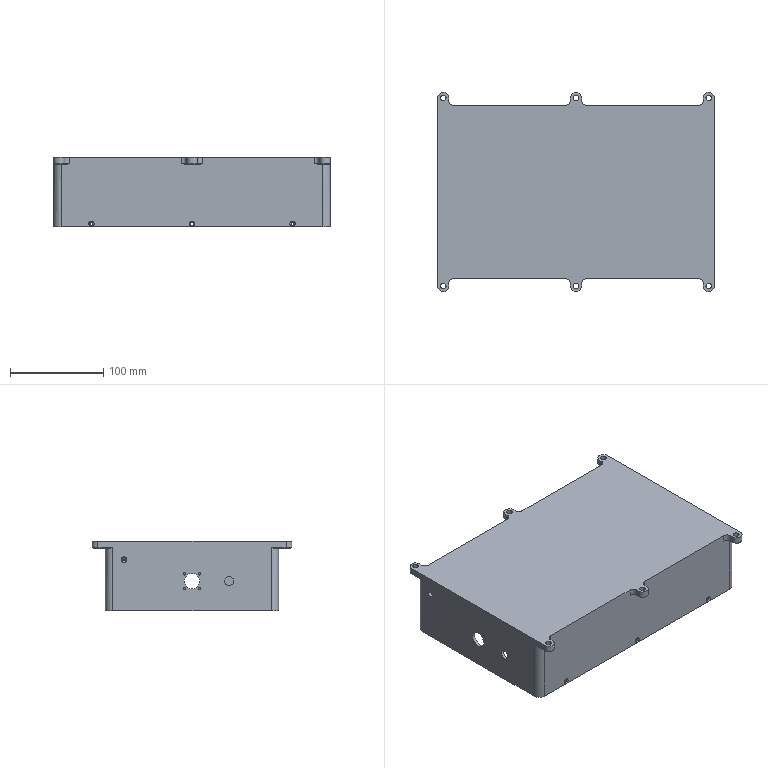NC program | NX | posted with a generic post | part box 297 x 214 x 75 mm
Whole program:
N10 G17 G21 G94 G90
(CAVITY_MILL , TOOL : D10JING)
N12 T14 M6
N14 G54
N16 G17 G0 G90 X-129.632 Y102.849 B0. C0. S9500 M3
N18 G43 Z30. H14
N20 Z-1.
N22 G94 G1 X-131.013 Y102.026 F1600.
N24 G3 X-131.501 Y101.153 R1.
N26 G1 X-131.5 Y101.
N28 Y98.
N30 X-128.347
N32 G3 X-127.481 Y98.5 R1.
N34 G1 X-126.615 Y100.
N36 G0 X-129.632 Y102.849 Z-2.
N38 G1 X-131.013 Y102.026
N40 G3 X-131.501 Y101.153 R1.
N42 G1 X-131.5 Y101.
N44 Y98.
N46 X-128.347
N48 G3 X-127.481 Y98.5 R1.
N50 G1 X-126.615 Y100.
N52 G0 X-129.632 Y102.849 Z-3.
N54 G1 X-131.013 Y102.026
N56 G3 X-131.501 Y101.153 R1.
N58 G1 X-131.5 Y101.
N60 Y98.
N62 X-128.347
N64 G3 X-127.481 Y98.5 R1.
N66 G1 X-126.615 Y100.
N68 G0 X-129.632 Y102.849 Z-4.
N70 G1 X-131.013 Y102.026
N72 G3 X-131.501 Y101.153 R1.
N74 G1 X-131.5 Y101.
N76 Y98.
N78 X-128.347
N80 G3 X-127.481 Y98.5 R1.
N82 G1 X-126.615 Y100.
N84 G0 X-129.632 Y102.849 Z-5.
N86 G1 X-131.013 Y102.026
N88 G3 X-131.501 Y101.153 R1.
N90 G1 X-131.5 Y101.
N92 Y98.
N94 X-128.347
N96 G3 X-127.481 Y98.5 R1.
N98 G1 X-126.615 Y100.
N100 G0 X-129.632 Y102.849 Z-6.
N102 G1 X-131.013 Y102.026
N104 G3 X-131.501 Y101.153 R1.
N106 G1 X-131.5 Y101.
N108 Y98.
N110 X-128.347
N112 G3 X-127.481 Y98.5 R1.
N114 G1 X-126.615 Y100.
N116 G0 X-129.632 Y102.849 Z-7.
N118 G1 X-131.013 Y102.026
N120 G3 X-131.501 Y101.153 R1.
N122 G1 X-131.5 Y101.
N124 Y98.
N126 X-128.347
N128 G3 X-127.481 Y98.5 R1.
N130 G1 X-126.615 Y100.
N132 G0 X-129.632 Y102.849 Z-8.
N134 G1 X-131.013 Y102.026
N136 G3 X-131.501 Y101.153 R1.
N138 G1 X-131.5 Y101.
N140 Y98.
N142 X-128.347
N144 G3 X-127.481 Y98.5 R1.
N146 G1 X-126.615 Y100.
N148 G0 X-129.632 Y102.849 Z-9.
N150 G1 X-131.013 Y102.026
N152 G3 X-131.501 Y101.153 R1.
N154 G1 X-131.5 Y101.
N156 Y98.
N158 X-128.347
N160 G3 X-127.481 Y98.5 R1.
N162 G1 X-126.615 Y100.
N164 G0 X-129.632 Y102.849 Z-10.
N166 G1 X-131.013 Y102.026
N168 G3 X-131.501 Y101.153 R1.
N170 G1 X-131.5 Y101.
N172 Y98.
N174 X-128.347
N176 G3 X-127.481 Y98.5 R1.
N178 G1 X-126.615 Y100.
N180 G0 Z30.
N182 X-15.885
N184 Z-1.
N186 G1 X-15.019 Y98.5
N188 G3 X-14.153 Y98. R1.
N190 G1 X-11.
N192 Y101.
N194 X-10.999 Y101.153
N196 G3 X-11.487 Y102.026 R1.
N198 G1 X-12.868 Y102.849
N200 G0 X-15.885 Y100. Z-2.
N202 G1 X-15.019 Y98.5
N204 G3 X-14.153 Y98. R1.
N206 G1 X-11.
N208 Y101.
N210 X-10.999 Y101.153
N212 G3 X-11.487 Y102.026 R1.
N214 G1 X-12.868 Y102.849
N216 G0 X-15.885 Y100. Z-3.
N218 G1 X-15.019 Y98.5
N220 G3 X-14.153 Y98. R1.
N222 G1 X-11.
N224 Y101.
N226 X-10.999 Y101.153
N228 G3 X-11.487 Y102.026 R1.
N230 G1 X-12.868 Y102.849
N232 G0 X-15.885 Y100. Z-4.
N234 G1 X-15.019 Y98.5
N236 G3 X-14.153 Y98. R1.
N238 G1 X-11.
N240 Y101.
N242 X-10.999 Y101.153
N244 G3 X-11.487 Y102.026 R1.
N246 G1 X-12.868 Y102.849
N248 G0 X-15.885 Y100. Z-5.
N250 G1 X-15.019 Y98.5
N252 G3 X-14.153 Y98. R1.
N254 G1 X-11.
N256 Y101.
N258 X-10.999 Y101.153
N260 G3 X-11.487 Y102.026 R1.
N262 G1 X-12.868 Y102.849
N264 G0 X-15.885 Y100. Z-6.
N266 G1 X-15.019 Y98.5
N268 G3 X-14.153 Y98. R1.
N270 G1 X-11.
N272 Y101.
N274 X-10.999 Y101.153
N276 G3 X-11.487 Y102.026 R1.
N278 G1 X-12.868 Y102.849
N280 G0 X-15.885 Y100. Z-7.
N282 G1 X-15.019 Y98.5
N284 G3 X-14.153 Y98. R1.
N286 G1 X-11.
N288 Y101.
N290 X-10.999 Y101.153
N292 G3 X-11.487 Y102.026 R1.
N294 G1 X-12.868 Y102.849
N296 G0 X-15.885 Y100. Z-8.
N298 G1 X-15.019 Y98.5
N300 G3 X-14.153 Y98. R1.
N302 G1 X-11.
N304 Y101.
N306 X-10.999 Y101.153
N308 G3 X-11.487 Y102.026 R1.
N310 G1 X-12.868 Y102.849
N312 G0 X-15.885 Y100. Z-9.
N314 G1 X-15.019 Y98.5
N316 G3 X-14.153 Y98. R1.
N318 G1 X-11.
N320 Y101.
N322 X-10.999 Y101.153
N324 G3 X-11.487 Y102.026 R1.
N326 G1 X-12.868 Y102.849
N328 G0 X-15.885 Y100. Z-10.
N330 G1 X-15.019 Y98.5
N332 G3 X-14.153 Y98. R1.
N334 G1 X-11.
N336 Y101.
N338 X-10.999 Y101.153
N340 G3 X-11.487 Y102.026 R1.
N342 G1 X-12.868 Y102.849
N344 G0 Z30.
N346 X12.868
N348 Z-1.
N350 G1 X11.487 Y102.026
N352 G3 X10.999 Y101.153 R1.
N354 G1 X11. Y101.
N356 Y98.
N358 X14.153
N360 G3 X15.019 Y98.5 R1.
N362 G1 X15.885 Y100.
N364 G0 X12.868 Y102.849 Z-2.
N366 G1 X11.487 Y102.026
N368 G3 X10.999 Y101.153 R1.
N370 G1 X11. Y101.
N372 Y98.
N374 X14.153
N376 G3 X15.019 Y98.5 R1.
N378 G1 X15.885 Y100.
N380 G0 X12.868 Y102.849 Z-3.
N382 G1 X11.487 Y102.026
N384 G3 X10.999 Y101.153 R1.
N386 G1 X11. Y101.
N388 Y98.
N390 X14.153
N392 G3 X15.019 Y98.5 R1.
N394 G1 X15.885 Y100.
N396 G0 X12.868 Y102.849 Z-4.
N398 G1 X11.487 Y102.026
N400 G3 X10.999 Y101.153 R1.
N402 G1 X11. Y101.
N404 Y98.
N406 X14.153
N408 G3 X15.019 Y98.5 R1.
N410 G1 X15.885 Y100.
N412 G0 X12.868 Y102.849 Z-5.
N414 G1 X11.487 Y102.026
N416 G3 X10.999 Y101.153 R1.
N418 G1 X11. Y101.
N420 Y98.
N422 X14.153
N424 G3 X15.019 Y98.5 R1.
N426 G1 X15.885 Y100.
N428 G0 X12.868 Y102.849 Z-6.
N430 G1 X11.487 Y102.026
N432 G3 X10.999 Y101.153 R1.
N434 G1 X11. Y101.
N436 Y98.
N438 X14.153
N440 G3 X15.019 Y98.5 R1.
N442 G1 X15.885 Y100.
N444 G0 X12.868 Y102.849 Z-7.
N446 G1 X11.487 Y102.026
N448 G3 X10.999 Y101.153 R1.
N450 G1 X11. Y101.
N452 Y98.
N454 X14.153
N456 G3 X15.019 Y98.5 R1.
N458 G1 X15.885 Y100.
N460 G0 X12.868 Y102.849 Z-8.
N462 G1 X11.487 Y102.026
N464 G3 X10.999 Y101.153 R1.
N466 G1 X11. Y101.
N468 Y98.
N470 X14.153
N472 G3 X15.019 Y98.5 R1.
N474 G1 X15.885 Y100.
N476 G0 X12.868 Y102.849 Z-9.
N478 G1 X11.487 Y102.026
N480 G3 X10.999 Y101.153 R1.
N482 G1 X11. Y101.
N484 Y98.
N486 X14.153
N488 G3 X15.019 Y98.5 R1.
N490 G1 X15.885 Y100.
N492 G0 X12.868 Y102.849 Z-10.
N494 G1 X11.487 Y102.026
N496 G3 X10.999 Y101.153 R1.
N498 G1 X11. Y101.
N500 Y98.
N502 X14.153
N504 G3 X15.019 Y98.5 R1.
N506 G1 X15.885 Y100.
N508 G0 Z30.
N510 X126.615
N512 Z-1.
N514 G1 X127.481 Y98.5
N516 G3 X128.347 Y98. R1.
N518 G1 X131.5
N520 Y101.
N522 X131.501 Y101.153
N524 G3 X131.013 Y102.026 R1.
N526 G1 X129.632 Y102.849
N528 G0 X126.615 Y100. Z-2.
N530 G1 X127.481 Y98.5
N532 G3 X128.347 Y98. R1.
N534 G1 X131.5
N536 Y101.
N538 X131.501 Y101.153
N540 G3 X131.013 Y102.026 R1.
N542 G1 X129.632 Y102.849
N544 G0 X126.615 Y100. Z-3.
N546 G1 X127.481 Y98.5
N548 G3 X128.347 Y98. R1.
N550 G1 X131.5
N552 Y101.
N554 X131.501 Y101.153
N556 G3 X131.013 Y102.026 R1.
N558 G1 X129.632 Y102.849
N560 G0 X126.615 Y100. Z-4.
N562 G1 X127.481 Y98.5
N564 G3 X128.347 Y98. R1.
N566 G1 X131.5
N568 Y101.
N570 X131.501 Y101.153
N572 G3 X131.013 Y102.026 R1.
N574 G1 X129.632 Y102.849
N576 G0 X126.615 Y100. Z-5.
N578 G1 X127.481 Y98.5
N580 G3 X128.347 Y98. R1.
N582 G1 X131.5
N584 Y101.
N586 X131.501 Y101.153
N588 G3 X131.013 Y102.026 R1.
N590 G1 X129.632 Y102.849
N592 G0 X126.615 Y100. Z-6.
N594 G1 X127.481 Y98.5
N596 G3 X128.347 Y98. R1.
N598 G1 X131.5
N600 Y101.
N602 X131.501 Y101.153
N604 G3 X131.013 Y102.026 R1.
N606 G1 X129.632 Y102.849
N608 G0 X126.615 Y100. Z-7.
N610 G1 X127.481 Y98.5
N612 G3 X128.347 Y98. R1.
N614 G1 X131.5
N616 Y101.
N618 X131.501 Y101.153
N620 G3 X131.013 Y102.026 R1.
N622 G1 X129.632 Y102.849
N624 G0 X126.615 Y100. Z-8.
N626 G1 X127.481 Y98.5
N628 G3 X128.347 Y98. R1.
N630 G1 X131.5
N632 Y101.
N634 X131.501 Y101.153
N636 G3 X131.013 Y102.026 R1.
N638 G1 X129.632 Y102.849
N640 G0 X126.615 Y100. Z-9.
N642 G1 X127.481 Y98.5
N644 G3 X128.347 Y98. R1.
N646 G1 X131.5
N648 Y101.
N650 X131.501 Y101.153
N652 G3 X131.013 Y102.026 R1.
N654 G1 X129.632 Y102.849
N656 G0 X126.615 Y100. Z-10.
N658 G1 X127.481 Y98.5
N660 G3 X128.347 Y98. R1.
N662 G1 X131.5
N664 Y101.
N666 X131.501 Y101.153
N668 G3 X131.013 Y102.026 R1.
N670 G1 X129.632 Y102.849
N672 G0 Z30.
N674 Y-102.849
N676 Z-1.
N678 G1 X131.013 Y-102.026
N680 G3 X131.501 Y-101.153 R1.
N682 G1 X131.5 Y-101.
N684 Y-98.
N686 X128.347
N688 G3 X127.481 Y-98.5 R1.
N690 G1 X126.615 Y-100.
N692 G0 X129.632 Y-102.849 Z-2.
N694 G1 X131.013 Y-102.026
N696 G3 X131.501 Y-101.153 R1.
N698 G1 X131.5 Y-101.
N700 Y-98.
N702 X128.347
N704 G3 X127.481 Y-98.5 R1.
N706 G1 X126.615 Y-100.
N708 G0 X129.632 Y-102.849 Z-3.
N710 G1 X131.013 Y-102.026
N712 G3 X131.501 Y-101.153 R1.
N714 G1 X131.5 Y-101.
N716 Y-98.
N718 X128.347
N720 G3 X127.481 Y-98.5 R1.
N722 G1 X126.615 Y-100.
N724 G0 X129.632 Y-102.849 Z-4.
N726 G1 X131.013 Y-102.026
N728 G3 X131.501 Y-101.153 R1.
N730 G1 X131.5 Y-101.
N732 Y-98.
N734 X128.347
N736 G3 X127.481 Y-98.5 R1.
N738 G1 X126.615 Y-100.
N740 G0 X129.632 Y-102.849 Z-5.
N742 G1 X131.013 Y-102.026
N744 G3 X131.501 Y-101.153 R1.
N746 G1 X131.5 Y-101.
N748 Y-98.
N750 X128.347
N752 G3 X127.481 Y-98.5 R1.
N754 G1 X126.615 Y-100.
N756 G0 X129.632 Y-102.849 Z-6.
N758 G1 X131.013 Y-102.026
N760 G3 X131.501 Y-101.153 R1.
N762 G1 X131.5 Y-101.
N764 Y-98.
N766 X128.347
N768 G3 X127.481 Y-98.5 R1.
N770 G1 X126.615 Y-100.
N772 G0 X129.632 Y-102.849 Z-7.
N774 G1 X131.013 Y-102.026
N776 G3 X131.501 Y-101.153 R1.
N778 G1 X131.5 Y-101.
N780 Y-98.
N782 X128.347
N784 G3 X127.481 Y-98.5 R1.
N786 G1 X126.615 Y-100.
N788 G0 X129.632 Y-102.849 Z-8.
N790 G1 X131.013 Y-102.026
N792 G3 X131.501 Y-101.153 R1.
N794 G1 X131.5 Y-101.
N796 Y-98.
N798 X128.347
N800 G3 X127.481 Y-98.5 R1.
N802 G1 X126.615 Y-100.
N804 G0 X129.632 Y-102.849 Z-9.
N806 G1 X131.013 Y-102.026
N808 G3 X131.501 Y-101.153 R1.
N810 G1 X131.5 Y-101.
N812 Y-98.
N814 X128.347
N816 G3 X127.481 Y-98.5 R1.
N818 G1 X126.615 Y-100.
N820 G0 X129.632 Y-102.849 Z-10.
N822 G1 X131.013 Y-102.026
N824 G3 X131.501 Y-101.153 R1.
N826 G1 X131.5 Y-101.
N828 Y-98.
N830 X128.347
N832 G3 X127.481 Y-98.5 R1.
N834 G1 X126.615 Y-100.
N836 G0 Z30.
N838 X15.885
N840 Z-1.
N842 G1 X15.019 Y-98.5
N844 G3 X14.153 Y-98. R1.
N846 G1 X11.
N848 Y-101.
N850 X10.999 Y-101.153
N852 G3 X11.487 Y-102.026 R1.
N854 G1 X12.868 Y-102.849
N856 G0 X15.885 Y-100. Z-2.
N858 G1 X15.019 Y-98.5
N860 G3 X14.153 Y-98. R1.
N862 G1 X11.
N864 Y-101.
N866 X10.999 Y-101.153
N868 G3 X11.487 Y-102.026 R1.
N870 G1 X12.868 Y-102.849
N872 G0 X15.885 Y-100. Z-3.
N874 G1 X15.019 Y-98.5
N876 G3 X14.153 Y-98. R1.
N878 G1 X11.
N880 Y-101.
N882 X10.999 Y-101.153
N884 G3 X11.487 Y-102.026 R1.
N886 G1 X12.868 Y-102.849
N888 G0 X15.885 Y-100. Z-4.
N890 G1 X15.019 Y-98.5
N892 G3 X14.153 Y-98. R1.
N894 G1 X11.
N896 Y-101.
N898 X10.999 Y-101.153
N900 G3 X11.487 Y-102.026 R1.
N902 G1 X12.868 Y-102.849
N904 G0 X15.885 Y-100. Z-5.
N906 G1 X15.019 Y-98.5
N908 G3 X14.153 Y-98. R1.
N910 G1 X11.
N912 Y-101.
N914 X10.999 Y-101.153
N916 G3 X11.487 Y-102.026 R1.
N918 G1 X12.868 Y-102.849
N920 G0 X15.885 Y-100. Z-6.
N922 G1 X15.019 Y-98.5
N924 G3 X14.153 Y-98. R1.
N926 G1 X11.
N928 Y-101.
N930 X10.999 Y-101.153
N932 G3 X11.487 Y-102.026 R1.
N934 G1 X12.868 Y-102.849
N936 G0 X15.885 Y-100. Z-7.
N938 G1 X15.019 Y-98.5
N940 G3 X14.153 Y-98. R1.
N942 G1 X11.
N944 Y-101.
N946 X10.999 Y-101.153
N948 G3 X11.487 Y-102.026 R1.
N950 G1 X12.868 Y-102.849
N952 G0 X15.885 Y-100. Z-8.
N954 G1 X15.019 Y-98.5
N956 G3 X14.153 Y-98. R1.
N958 G1 X11.
N960 Y-101.
N962 X10.999 Y-101.153
N964 G3 X11.487 Y-102.026 R1.
N966 G1 X12.868 Y-102.849
N968 G0 X15.885 Y-100. Z-9.
N970 G1 X15.019 Y-98.5
N972 G3 X14.153 Y-98. R1.
N974 G1 X11.
N976 Y-101.
N978 X10.999 Y-101.153
N980 G3 X11.487 Y-102.026 R1.
N982 G1 X12.868 Y-102.849
N984 G0 X15.885 Y-100. Z-10.
N986 G1 X15.019 Y-98.5
N988 G3 X14.153 Y-98. R1.
N990 G1 X11.
N992 Y-101.
N994 X10.999 Y-101.153
N996 G3 X11.487 Y-102.026 R1.
N998 G1 X12.868 Y-102.849
N1000 G0 Z30.
N1002 X-12.868
N1004 Z-1.
N1006 G1 X-11.487 Y-102.026
N1008 G3 X-10.999 Y-101.153 R1.
N1010 G1 X-11. Y-101.
N1012 Y-98.
N1014 X-14.153
N1016 G3 X-15.019 Y-98.5 R1.
N1018 G1 X-15.885 Y-100.
N1020 G0 X-12.868 Y-102.849 Z-2.
N1022 G1 X-11.487 Y-102.026
N1024 G3 X-10.999 Y-101.153 R1.
N1026 G1 X-11. Y-101.
N1028 Y-98.
N1030 X-14.153
N1032 G3 X-15.019 Y-98.5 R1.
N1034 G1 X-15.885 Y-100.
N1036 G0 X-12.868 Y-102.849 Z-3.
N1038 G1 X-11.487 Y-102.026
N1040 G3 X-10.999 Y-101.153 R1.
N1042 G1 X-11. Y-101.
N1044 Y-98.
N1046 X-14.153
N1048 G3 X-15.019 Y-98.5 R1.
N1050 G1 X-15.885 Y-100.
N1052 G0 X-12.868 Y-102.849 Z-4.
N1054 G1 X-11.487 Y-102.026
N1056 G3 X-10.999 Y-101.153 R1.
N1058 G1 X-11. Y-101.
N1060 Y-98.
N1062 X-14.153
N1064 G3 X-15.019 Y-98.5 R1.
N1066 G1 X-15.885 Y-100.
N1068 G0 X-12.868 Y-102.849 Z-5.
N1070 G1 X-11.487 Y-102.026
N1072 G3 X-10.999 Y-101.153 R1.
N1074 G1 X-11. Y-101.
N1076 Y-98.
N1078 X-14.153
N1080 G3 X-15.019 Y-98.5 R1.
N1082 G1 X-15.885 Y-100.
N1084 G0 X-12.868 Y-102.849 Z-6.
N1086 G1 X-11.487 Y-102.026
N1088 G3 X-10.999 Y-101.153 R1.
N1090 G1 X-11. Y-101.
N1092 Y-98.
N1094 X-14.153
N1096 G3 X-15.019 Y-98.5 R1.
N1098 G1 X-15.885 Y-100.
N1100 G0 X-12.868 Y-102.849 Z-7.
N1102 G1 X-11.487 Y-102.026
N1104 G3 X-10.999 Y-101.153 R1.
N1106 G1 X-11. Y-101.
N1108 Y-98.
N1110 X-14.153
N1112 G3 X-15.019 Y-98.5 R1.
N1114 G1 X-15.885 Y-100.
N1116 G0 X-12.868 Y-102.849 Z-8.
N1118 G1 X-11.487 Y-102.026
N1120 G3 X-10.999 Y-101.153 R1.
N1122 G1 X-11. Y-101.
N1124 Y-98.
N1126 X-14.153
N1128 G3 X-15.019 Y-98.5 R1.
N1130 G1 X-15.885 Y-100.
N1132 G0 X-12.868 Y-102.849 Z-9.
N1134 G1 X-11.487 Y-102.026
N1136 G3 X-10.999 Y-101.153 R1.
N1138 G1 X-11. Y-101.
N1140 Y-98.
N1142 X-14.153
N1144 G3 X-15.019 Y-98.5 R1.
N1146 G1 X-15.885 Y-100.
N1148 G0 X-12.868 Y-102.849 Z-10.
N1150 G1 X-11.487 Y-102.026
N1152 G3 X-10.999 Y-101.153 R1.
N1154 G1 X-11. Y-101.
N1156 Y-98.
N1158 X-14.153
N1160 G3 X-15.019 Y-98.5 R1.
N1162 G1 X-15.885 Y-100.
N1164 G0 Z30.
N1166 X-126.615
N1168 Z-1.
N1170 G1 X-127.481 Y-98.5
N1172 G3 X-128.347 Y-98. R1.
N1174 G1 X-131.5
N1176 Y-101.
N1178 X-131.501 Y-101.153
N1180 G3 X-131.013 Y-102.026 R1.
N1182 G1 X-129.632 Y-102.849
N1184 G0 X-126.615 Y-100. Z-2.
N1186 G1 X-127.481 Y-98.5
N1188 G3 X-128.347 Y-98. R1.
N1190 G1 X-131.5
N1192 Y-101.
N1194 X-131.501 Y-101.153
N1196 G3 X-131.013 Y-102.026 R1.
N1198 G1 X-129.632 Y-102.849
N1200 G0 X-126.615 Y-100. Z-3.
N1202 G1 X-127.481 Y-98.5
N1204 G3 X-128.347 Y-98. R1.
N1206 G1 X-131.5
N1208 Y-101.
N1210 X-131.501 Y-101.153
N1212 G3 X-131.013 Y-102.026 R1.
N1214 G1 X-129.632 Y-102.849
N1216 G0 X-126.615 Y-100. Z-4.
N1218 G1 X-127.481 Y-98.5
N1220 G3 X-128.347 Y-98. R1.
N1222 G1 X-131.5
N1224 Y-101.
N1226 X-131.501 Y-101.153
N1228 G3 X-131.013 Y-102.026 R1.
N1230 G1 X-129.632 Y-102.849
N1232 G0 X-126.615 Y-100. Z-5.
N1234 G1 X-127.481 Y-98.5
N1236 G3 X-128.347 Y-98. R1.
N1238 G1 X-131.5
N1240 Y-101.
N1242 X-131.501 Y-101.153
N1244 G3 X-131.013 Y-102.026 R1.
N1246 G1 X-129.632 Y-102.849
N1248 G0 X-126.615 Y-100. Z-6.
N1250 G1 X-127.481 Y-98.5
N1252 G3 X-128.347 Y-98. R1.
N1254 G1 X-131.5
N1256 Y-101.
N1258 X-131.501 Y-101.153
N1260 G3 X-131.013 Y-102.026 R1.
N1262 G1 X-129.632 Y-102.849
N1264 G0 X-126.615 Y-100. Z-7.
N1266 G1 X-127.481 Y-98.5
N1268 G3 X-128.347 Y-98. R1.
N1270 G1 X-131.5
N1272 Y-101.
N1274 X-131.501 Y-101.153
N1276 G3 X-131.013 Y-102.026 R1.
N1278 G1 X-129.632 Y-102.849
N1280 G0 X-126.615 Y-100. Z-8.
N1282 G1 X-127.481 Y-98.5
N1284 G3 X-128.347 Y-98. R1.
N1286 G1 X-131.5
N1288 Y-101.
N1290 X-131.501 Y-101.153
N1292 G3 X-131.013 Y-102.026 R1.
N1294 G1 X-129.632 Y-102.849
N1296 G0 X-126.615 Y-100. Z-9.
N1298 G1 X-127.481 Y-98.5
N1300 G3 X-128.347 Y-98. R1.
N1302 G1 X-131.5
N1304 Y-101.
N1306 X-131.501 Y-101.153
N1308 G3 X-131.013 Y-102.026 R1.
N1310 G1 X-129.632 Y-102.849
N1312 G0 X-126.615 Y-100. Z-10.
N1314 G1 X-127.481 Y-98.5
N1316 G3 X-128.347 Y-98. R1.
N1318 G1 X-131.5
N1320 Y-101.
N1322 X-131.501 Y-101.153
N1324 G3 X-131.013 Y-102.026 R1.
N1326 G1 X-129.632 Y-102.849
N1328 G0 Z30.
N1330 M5
N1332 M2